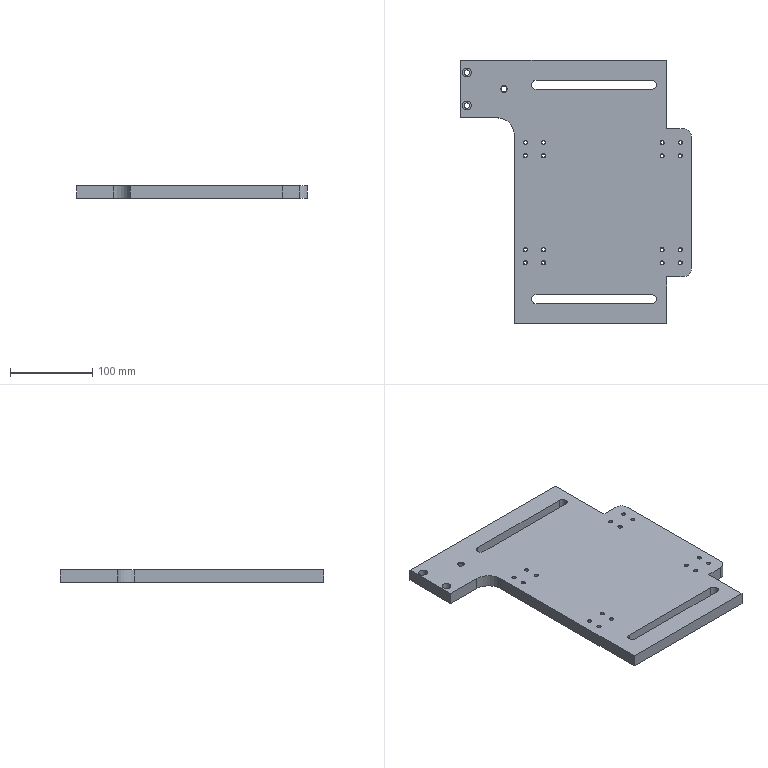Part | STEP file | YBQDJ-SSJ-1 | 1 solid | 81 faces | box 280 x 320 x 15 mm | volume 982860 mm3 | cone 35 | cylinder 28 | plane 18 | commonest cylinder face diameters 4.2 x16 11 x4 6.5 x2 10.7 x2 20 x2 6.8 x1